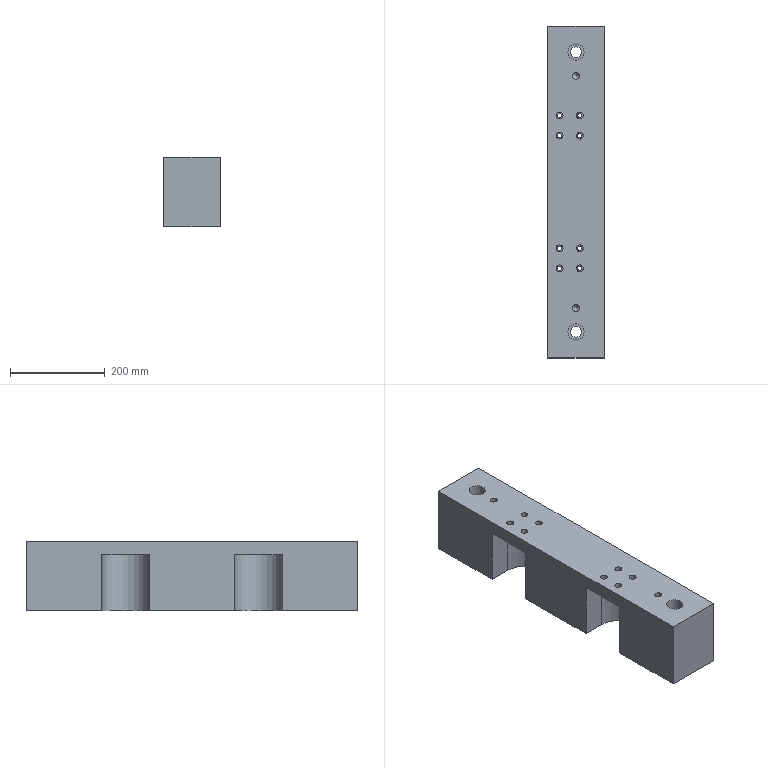Part | STEP file | lll_id2466_x_t | 1 solid | 48 faces | box 120 x 700 x 147.5 mm | volume 10097568 mm3 | cylinder 24 | plane 22 | cone 2 | commonest cylinder face diameters 9.009 x8 14.508 x8 14.506 x2 23.009 x2 34.008 x2 100 x2
STEP:
#1=CARTESIAN_POINT('',(1753.439,295.,370.));
#2=VERTEX_POINT('',#1);
#3=CARTESIAN_POINT('',(1736.435,295.,370.));
#4=DIRECTION('',(0.,0.,-1.));
#5=DIRECTION('',(1.,0.,0.));
#6=AXIS2_PLACEMENT_3D('',#3,#4,#5);
#7=CIRCLE('',#6,17.004);
#8=EDGE_CURVE('',#2,#2,#7,.T.);
#9=ORIENTED_EDGE('',*,*,#8,.T.);
#10=EDGE_LOOP('',(#9));
#11=FACE_BOUND('',#10,.T.);
#12=CARTESIAN_POINT('',(1753.439,-295.,370.));
#13=VERTEX_POINT('',#12);
#14=CARTESIAN_POINT('',(1736.435,-295.,370.));
#15=DIRECTION('',(0.,0.,-1.));
#16=DIRECTION('',(1.,0.,0.));
#17=AXIS2_PLACEMENT_3D('',#14,#15,#16);
#18=CIRCLE('',#17,17.004);
#19=EDGE_CURVE('',#13,#13,#18,.T.);
#20=ORIENTED_EDGE('',*,*,#19,.T.);
#21=EDGE_LOOP('',(#20));
#22=FACE_BOUND('',#21,.T.);
#23=CARTESIAN_POINT('',(1709.041,118.787,370.));
#24=VERTEX_POINT('',#23);
#25=CARTESIAN_POINT('',(1701.787,118.787,370.));
#26=DIRECTION('',(0.,0.,-1.));
#27=DIRECTION('',(1.,0.,0.));
#28=AXIS2_PLACEMENT_3D('',#25,#26,#27);
#29=CIRCLE('',#28,7.254);
#30=EDGE_CURVE('',#24,#24,#29,.T.);
#31=ORIENTED_EDGE('',*,*,#30,.T.);
#32=EDGE_LOOP('',(#31));
#33=FACE_BOUND('',#32,.T.);
#34=CARTESIAN_POINT('',(1751.467,118.787,370.));
#35=VERTEX_POINT('',#34);
#36=CARTESIAN_POINT('',(1744.213,118.787,370.));
#37=DIRECTION('',(0.,0.,-1.));
#38=DIRECTION('',(1.,0.,0.));
#39=AXIS2_PLACEMENT_3D('',#36,#37,#38);
#40=CIRCLE('',#39,7.254);
#41=EDGE_CURVE('',#35,#35,#40,.T.);
#42=ORIENTED_EDGE('',*,*,#41,.T.);
#43=EDGE_LOOP('',(#42));
#44=FACE_BOUND('',#43,.T.);
#45=CARTESIAN_POINT('',(1751.467,-118.787,370.));
#46=VERTEX_POINT('',#45);
#47=CARTESIAN_POINT('',(1744.213,-118.787,370.));
#48=DIRECTION('',(0.,0.,-1.));
#49=DIRECTION('',(1.,0.,0.));
#50=AXIS2_PLACEMENT_3D('',#47,#48,#49);
#51=CIRCLE('',#50,7.254);
#52=EDGE_CURVE('',#46,#46,#51,.T.);
#53=ORIENTED_EDGE('',*,*,#52,.T.);
#54=EDGE_LOOP('',(#53));
#55=FACE_BOUND('',#54,.T.);
#56=CARTESIAN_POINT('',(1709.041,-118.787,370.));
#57=VERTEX_POINT('',#56);
#58=CARTESIAN_POINT('',(1701.787,-118.787,370.));
#59=DIRECTION('',(0.,0.,-1.));
#60=DIRECTION('',(1.,0.,0.));
#61=AXIS2_PLACEMENT_3D('',#58,#59,#60);
#62=CIRCLE('',#61,7.254);
#63=EDGE_CURVE('',#57,#57,#62,.T.);
#64=ORIENTED_EDGE('',*,*,#63,.T.);
#65=EDGE_LOOP('',(#64));
#66=FACE_BOUND('',#65,.T.);
#67=CARTESIAN_POINT('',(1751.467,161.213,370.));
#68=VERTEX_POINT('',#67);
#69=CARTESIAN_POINT('',(1744.213,161.213,370.));
#70=DIRECTION('',(0.,0.,-1.));
#71=DIRECTION('',(1.,0.,0.));
#72=AXIS2_PLACEMENT_3D('',#69,#70,#71);
#73=CIRCLE('',#72,7.254);
#74=EDGE_CURVE('',#68,#68,#73,.T.);
#75=ORIENTED_EDGE('',*,*,#74,.T.);
#76=EDGE_LOOP('',(#75));
#77=FACE_BOUND('',#76,.T.);
#78=CARTESIAN_POINT('',(1709.041,-161.213,370.));
#79=VERTEX_POINT('',#78);
#80=CARTESIAN_POINT('',(1701.787,-161.213,370.));
#81=DIRECTION('',(0.,0.,-1.));
#82=DIRECTION('',(1.,0.,0.));
#83=AXIS2_PLACEMENT_3D('',#80,#81,#82);
#84=CIRCLE('',#83,7.254);
#85=EDGE_CURVE('',#79,#79,#84,.T.);
#86=ORIENTED_EDGE('',*,*,#85,.T.);
#87=EDGE_LOOP('',(#86));
#88=FACE_BOUND('',#87,.T.);
#89=CARTESIAN_POINT('',(1751.467,-161.213,370.));
#90=VERTEX_POINT('',#89);
#91=CARTESIAN_POINT('',(1744.213,-161.213,370.));
#92=DIRECTION('',(0.,0.,-1.));
#93=DIRECTION('',(1.,0.,0.));
#94=AXIS2_PLACEMENT_3D('',#91,#92,#93);
#95=CIRCLE('',#94,7.254);
#96=EDGE_CURVE('',#90,#90,#95,.T.);
#97=ORIENTED_EDGE('',*,*,#96,.T.);
#98=EDGE_LOOP('',(#97));
#99=FACE_BOUND('',#98,.T.);
#100=CARTESIAN_POINT('',(1709.041,161.213,370.));
#101=VERTEX_POINT('',#100);
#102=CARTESIAN_POINT('',(1701.787,161.213,370.));
#103=DIRECTION('',(0.,0.,-1.));
#104=DIRECTION('',(1.,0.,0.));
#105=AXIS2_PLACEMENT_3D('',#102,#103,#104);
#106=CIRCLE('',#105,7.254);
#107=EDGE_CURVE('',#101,#101,#106,.T.);
#108=ORIENTED_EDGE('',*,*,#107,.T.);
#109=EDGE_LOOP('',(#108));
#110=FACE_BOUND('',#109,.T.);
#111=CARTESIAN_POINT('',(1796.435,-350.,370.));
#112=VERTEX_POINT('',#111);
#113=CARTESIAN_POINT('',(1676.435,-350.,370.));
#114=VERTEX_POINT('',#113);
#115=CARTESIAN_POINT('',(3982.751,-350.,370.));
#116=DIRECTION('',(-1.,0.,0.));
#117=VECTOR('',#116,1.);
#118=LINE('',#115,#117);
#119=EDGE_CURVE('',#112,#114,#118,.T.);
#120=ORIENTED_EDGE('',*,*,#119,.F.);
#121=CARTESIAN_POINT('',(1796.435,350.,370.));
#122=VERTEX_POINT('',#121);
#123=CARTESIAN_POINT('',(1796.435,1.,370.));
#124=DIRECTION('',(0.,-1.,0.));
#125=VECTOR('',#124,1.);
#126=LINE('',#123,#125);
#127=EDGE_CURVE('',#122,#112,#126,.T.);
#128=ORIENTED_EDGE('',*,*,#127,.F.);
#129=CARTESIAN_POINT('',(1676.435,350.,370.));
#130=VERTEX_POINT('',#129);
#131=CARTESIAN_POINT('',(3982.751,350.,370.));
#132=DIRECTION('',(1.,0.,0.));
#133=VECTOR('',#132,1.);
#134=LINE('',#131,#133);
#135=EDGE_CURVE('',#130,#122,#134,.T.);
#136=ORIENTED_EDGE('',*,*,#135,.F.);
#137=CARTESIAN_POINT('',(1676.435,0.,370.));
#138=DIRECTION('',(0.,1.,0.));
#139=VECTOR('',#138,1.);
#140=LINE('',#137,#139);
#141=EDGE_CURVE('',#114,#130,#140,.T.);
#142=ORIENTED_EDGE('',*,*,#141,.F.);
#143=EDGE_LOOP('',(#120,#128,#136,#142));
#144=FACE_BOUND('',#143,.T.);
#145=CARTESIAN_POINT('',(1743.688,-245.,370.));
#146=VERTEX_POINT('',#145);
#147=CARTESIAN_POINT('',(1736.435,-245.,370.));
#148=DIRECTION('',(0.,0.,-1.));
#149=DIRECTION('',(1.,0.,0.));
#150=AXIS2_PLACEMENT_3D('',#147,#148,#149);
#151=CIRCLE('',#150,7.253);
#152=EDGE_CURVE('',#146,#146,#151,.T.);
#153=ORIENTED_EDGE('',*,*,#152,.T.);
#154=EDGE_LOOP('',(#153));
#155=FACE_BOUND('',#154,.T.);
#156=CARTESIAN_POINT('',(1743.688,245.,370.));
#157=VERTEX_POINT('',#156);
#158=CARTESIAN_POINT('',(1736.435,245.,370.));
#159=DIRECTION('',(0.,0.,1.));
#160=DIRECTION('',(1.,0.,0.));
#161=AXIS2_PLACEMENT_3D('',#158,#159,#160);
#162=CIRCLE('',#161,7.253);
#163=EDGE_CURVE('',#157,#157,#162,.T.);
#164=ORIENTED_EDGE('',*,*,#163,.F.);
#165=EDGE_LOOP('',(#164));
#166=FACE_BOUND('',#165,.T.);
#167=CARTESIAN_POINT('',(3982.751,1.,370.));
#168=DIRECTION('',(0.,0.,-1.));
#169=DIRECTION('',(-1.,0.,0.));
#170=AXIS2_PLACEMENT_3D('',#167,#168,#169);
#171=PLANE('',#170);
#172=ADVANCED_FACE('',(#11,#22,#33,#44,#55,#66,#77,#88,#99,#110,#144,#155,#166),#171,.F.);
#173=CARTESIAN_POINT('',(1706.291,161.213,341.));
#174=VERTEX_POINT('',#173);
#175=CARTESIAN_POINT('',(1701.787,161.213,341.));
#176=DIRECTION('',(0.,0.,1.));
#177=DIRECTION('',(1.,0.,0.));
#178=AXIS2_PLACEMENT_3D('',#175,#176,#177);
#179=CIRCLE('',#178,4.505);
#180=EDGE_CURVE('',#174,#174,#179,.T.);
#181=ORIENTED_EDGE('',*,*,#180,.T.);
#182=EDGE_LOOP('',(#181));
#183=FACE_BOUND('',#182,.T.);
#184=CARTESIAN_POINT('',(1748.718,161.213,341.));
#185=VERTEX_POINT('',#184);
#186=CARTESIAN_POINT('',(1744.213,161.213,341.));
#187=DIRECTION('',(0.,0.,1.));
#188=DIRECTION('',(1.,0.,0.));
#189=AXIS2_PLACEMENT_3D('',#186,#187,#188);
#190=CIRCLE('',#189,4.505);
#191=EDGE_CURVE('',#185,#185,#190,.T.);
#192=ORIENTED_EDGE('',*,*,#191,.T.);
#193=EDGE_LOOP('',(#192));
#194=FACE_BOUND('',#193,.T.);
#195=CARTESIAN_POINT('',(1748.718,118.787,341.));
#196=VERTEX_POINT('',#195);
#197=CARTESIAN_POINT('',(1744.213,118.787,341.));
#198=DIRECTION('',(0.,0.,1.));
#199=DIRECTION('',(1.,0.,0.));
#200=AXIS2_PLACEMENT_3D('',#197,#198,#199);
#201=CIRCLE('',#200,4.505);
#202=EDGE_CURVE('',#196,#196,#201,.T.);
#203=ORIENTED_EDGE('',*,*,#202,.T.);
#204=EDGE_LOOP('',(#203));
#205=FACE_BOUND('',#204,.T.);
#206=CARTESIAN_POINT('',(1706.291,118.787,341.));
#207=VERTEX_POINT('',#206);
#208=CARTESIAN_POINT('',(1701.787,118.787,341.));
#209=DIRECTION('',(0.,0.,1.));
#210=DIRECTION('',(1.,0.,0.));
#211=AXIS2_PLACEMENT_3D('',#208,#209,#210);
#212=CIRCLE('',#211,4.505);
#213=EDGE_CURVE('',#207,#207,#212,.T.);
#214=ORIENTED_EDGE('',*,*,#213,.T.);
#215=EDGE_LOOP('',(#214));
#216=FACE_BOUND('',#215,.T.);
#217=CARTESIAN_POINT('',(1723.,190.,341.));
#218=VERTEX_POINT('',#217);
#219=CARTESIAN_POINT('',(1676.435,190.,341.));
#220=VERTEX_POINT('',#219);
#221=CARTESIAN_POINT('',(1723.,190.,341.));
#222=DIRECTION('',(-1.,0.,0.));
#223=VECTOR('',#222,1.);
#224=LINE('',#221,#223);
#225=EDGE_CURVE('',#218,#220,#224,.T.);
#226=ORIENTED_EDGE('',*,*,#225,.F.);
#227=CARTESIAN_POINT('',(1723.,90.,341.));
#228=VERTEX_POINT('',#227);
#229=CARTESIAN_POINT('',(1723.,140.,341.));
#230=DIRECTION('',(0.,0.,1.));
#231=DIRECTION('',(1.,0.,0.));
#232=AXIS2_PLACEMENT_3D('',#229,#230,#231);
#233=CIRCLE('',#232,50.);
#234=EDGE_CURVE('',#228,#218,#233,.T.);
#235=ORIENTED_EDGE('',*,*,#234,.F.);
#236=CARTESIAN_POINT('',(1676.435,90.,341.));
#237=VERTEX_POINT('',#236);
#238=CARTESIAN_POINT('',(1723.,90.,341.));
#239=DIRECTION('',(-1.,0.,0.));
#240=VECTOR('',#239,1.);
#241=LINE('',#238,#240);
#242=EDGE_CURVE('',#228,#237,#241,.T.);
#243=ORIENTED_EDGE('',*,*,#242,.T.);
#244=CARTESIAN_POINT('',(1676.435,0.,341.));
#245=DIRECTION('',(0.,-1.,0.));
#246=VECTOR('',#245,1.);
#247=LINE('',#244,#246);
#248=EDGE_CURVE('',#220,#237,#247,.T.);
#249=ORIENTED_EDGE('',*,*,#248,.F.);
#250=EDGE_LOOP('',(#226,#235,#243,#249));
#251=FACE_BOUND('',#250,.T.);
#252=CARTESIAN_POINT('',(1723.,140.,341.));
#253=DIRECTION('',(0.,0.,1.));
#254=DIRECTION('',(1.,0.,0.));
#255=AXIS2_PLACEMENT_3D('',#252,#253,#254);
#256=PLANE('',#255);
#257=ADVANCED_FACE('',(#183,#194,#205,#216,#251),#256,.F.);
#258=CARTESIAN_POINT('',(1748.718,-161.213,341.));
#259=VERTEX_POINT('',#258);
#260=CARTESIAN_POINT('',(1744.213,-161.213,341.));
#261=DIRECTION('',(0.,0.,1.));
#262=DIRECTION('',(1.,0.,0.));
#263=AXIS2_PLACEMENT_3D('',#260,#261,#262);
#264=CIRCLE('',#263,4.505);
#265=EDGE_CURVE('',#259,#259,#264,.T.);
#266=ORIENTED_EDGE('',*,*,#265,.T.);
#267=EDGE_LOOP('',(#266));
#268=FACE_BOUND('',#267,.T.);
#269=CARTESIAN_POINT('',(1706.291,-161.213,341.));
#270=VERTEX_POINT('',#269);
#271=CARTESIAN_POINT('',(1701.787,-161.213,341.));
#272=DIRECTION('',(0.,0.,1.));
#273=DIRECTION('',(1.,0.,0.));
#274=AXIS2_PLACEMENT_3D('',#271,#272,#273);
#275=CIRCLE('',#274,4.505);
#276=EDGE_CURVE('',#270,#270,#275,.T.);
#277=ORIENTED_EDGE('',*,*,#276,.T.);
#278=EDGE_LOOP('',(#277));
#279=FACE_BOUND('',#278,.T.);
#280=CARTESIAN_POINT('',(1706.291,-118.787,341.));
#281=VERTEX_POINT('',#280);
#282=CARTESIAN_POINT('',(1701.787,-118.787,341.));
#283=DIRECTION('',(0.,0.,1.));
#284=DIRECTION('',(1.,0.,0.));
#285=AXIS2_PLACEMENT_3D('',#282,#283,#284);
#286=CIRCLE('',#285,4.505);
#287=EDGE_CURVE('',#281,#281,#286,.T.);
#288=ORIENTED_EDGE('',*,*,#287,.T.);
#289=EDGE_LOOP('',(#288));
#290=FACE_BOUND('',#289,.T.);
#291=CARTESIAN_POINT('',(1748.718,-118.787,341.));
#292=VERTEX_POINT('',#291);
#293=CARTESIAN_POINT('',(1744.213,-118.787,341.));
#294=DIRECTION('',(0.,0.,1.));
#295=DIRECTION('',(1.,0.,0.));
#296=AXIS2_PLACEMENT_3D('',#293,#294,#295);
#297=CIRCLE('',#296,4.505);
#298=EDGE_CURVE('',#292,#292,#297,.T.);
#299=ORIENTED_EDGE('',*,*,#298,.T.);
#300=EDGE_LOOP('',(#299));
#301=FACE_BOUND('',#300,.T.);
#302=CARTESIAN_POINT('',(1723.,-90.,341.));
#303=VERTEX_POINT('',#302);
#304=CARTESIAN_POINT('',(1676.435,-90.,341.));
#305=VERTEX_POINT('',#304);
#306=CARTESIAN_POINT('',(1723.,-90.,341.));
#307=DIRECTION('',(-1.,0.,0.));
#308=VECTOR('',#307,1.);
#309=LINE('',#306,#308);
#310=EDGE_CURVE('',#303,#305,#309,.T.);
#311=ORIENTED_EDGE('',*,*,#310,.F.);
#312=CARTESIAN_POINT('',(1723.,-190.,341.));
#313=VERTEX_POINT('',#312);
#314=CARTESIAN_POINT('',(1723.,-140.,341.));
#315=DIRECTION('',(0.,0.,1.));
#316=DIRECTION('',(1.,0.,0.));
#317=AXIS2_PLACEMENT_3D('',#314,#315,#316);
#318=CIRCLE('',#317,50.);
#319=EDGE_CURVE('',#313,#303,#318,.T.);
#320=ORIENTED_EDGE('',*,*,#319,.F.);
#321=CARTESIAN_POINT('',(1676.435,-190.,341.));
#322=VERTEX_POINT('',#321);
#323=CARTESIAN_POINT('',(1723.,-190.,341.));
#324=DIRECTION('',(-1.,0.,0.));
#325=VECTOR('',#324,1.);
#326=LINE('',#323,#325);
#327=EDGE_CURVE('',#313,#322,#326,.T.);
#328=ORIENTED_EDGE('',*,*,#327,.T.);
#329=CARTESIAN_POINT('',(1676.435,0.,341.));
#330=DIRECTION('',(0.,-1.,0.));
#331=VECTOR('',#330,1.);
#332=LINE('',#329,#331);
#333=EDGE_CURVE('',#305,#322,#332,.T.);
#334=ORIENTED_EDGE('',*,*,#333,.F.);
#335=EDGE_LOOP('',(#311,#320,#328,#334));
#336=FACE_BOUND('',#335,.T.);
#337=CARTESIAN_POINT('',(1723.,140.,341.));
#338=DIRECTION('',(0.,0.,1.));
#339=DIRECTION('',(1.,0.,0.));
#340=AXIS2_PLACEMENT_3D('',#337,#338,#339);
#341=PLANE('',#340);
#342=ADVANCED_FACE('',(#268,#279,#290,#301,#336),#341,.F.);
#343=CARTESIAN_POINT('',(1796.435,-350.,222.5));
#344=VERTEX_POINT('',#343);
#345=CARTESIAN_POINT('',(1796.435,-350.,310.));
#346=DIRECTION('',(0.,0.,-1.));
#347=VECTOR('',#346,1.);
#348=LINE('',#345,#347);
#349=EDGE_CURVE('',#112,#344,#348,.T.);
#350=ORIENTED_EDGE('',*,*,#349,.T.);
#351=CARTESIAN_POINT('',(1796.435,350.,222.5));
#352=VERTEX_POINT('',#351);
#353=CARTESIAN_POINT('',(1796.435,600.,222.5));
#354=DIRECTION('',(0.,-1.,0.));
#355=VECTOR('',#354,1.);
#356=LINE('',#353,#355);
#357=EDGE_CURVE('',#352,#344,#356,.T.);
#358=ORIENTED_EDGE('',*,*,#357,.F.);
#359=CARTESIAN_POINT('',(1796.435,350.,310.));
#360=DIRECTION('',(0.,0.,-1.));
#361=VECTOR('',#360,1.);
#362=LINE('',#359,#361);
#363=EDGE_CURVE('',#122,#352,#362,.T.);
#364=ORIENTED_EDGE('',*,*,#363,.F.);
#365=ORIENTED_EDGE('',*,*,#127,.T.);
#366=EDGE_LOOP('',(#350,#358,#364,#365));
#367=FACE_OUTER_BOUND('',#366,.T.);
#368=CARTESIAN_POINT('',(1796.435,600.,310.));
#369=DIRECTION('',(1.,0.,0.));
#370=DIRECTION('',(0.,0.,-1.));
#371=AXIS2_PLACEMENT_3D('',#368,#369,#370);
#372=PLANE('',#371);
#373=ADVANCED_FACE('',(#367),#372,.T.);
#374=CARTESIAN_POINT('',(1676.435,-350.,222.5));
#375=VERTEX_POINT('',#374);
#376=CARTESIAN_POINT('',(1676.435,-350.,241.25));
#377=DIRECTION('',(0.,0.,-1.));
#378=VECTOR('',#377,1.);
#379=LINE('',#376,#378);
#380=EDGE_CURVE('',#114,#375,#379,.T.);
#381=ORIENTED_EDGE('',*,*,#380,.T.);
#382=CARTESIAN_POINT('',(3982.751,-350.,222.5));
#383=DIRECTION('',(-1.,0.,0.));
#384=VECTOR('',#383,1.);
#385=LINE('',#382,#384);
#386=EDGE_CURVE('',#344,#375,#385,.T.);
#387=ORIENTED_EDGE('',*,*,#386,.F.);
#388=ORIENTED_EDGE('',*,*,#349,.F.);
#389=ORIENTED_EDGE('',*,*,#119,.T.);
#390=EDGE_LOOP('',(#381,#387,#388,#389));
#391=FACE_OUTER_BOUND('',#390,.T.);
#392=CARTESIAN_POINT('',(1796.435,-350.,310.));
#393=DIRECTION('',(0.,-1.,0.));
#394=DIRECTION('',(0.,0.,-1.));
#395=AXIS2_PLACEMENT_3D('',#392,#393,#394);
#396=PLANE('',#395);
#397=ADVANCED_FACE('',(#391),#396,.T.);
#398=ORIENTED_EDGE('',*,*,#363,.T.);
#399=CARTESIAN_POINT('',(1676.435,350.,222.5));
#400=VERTEX_POINT('',#399);
#401=CARTESIAN_POINT('',(3982.751,350.,222.5));
#402=DIRECTION('',(1.,0.,0.));
#403=VECTOR('',#402,1.);
#404=LINE('',#401,#403);
#405=EDGE_CURVE('',#400,#352,#404,.T.);
#406=ORIENTED_EDGE('',*,*,#405,.F.);
#407=CARTESIAN_POINT('',(1676.435,350.,241.25));
#408=DIRECTION('',(0.,0.,1.));
#409=VECTOR('',#408,1.);
#410=LINE('',#407,#409);
#411=EDGE_CURVE('',#400,#130,#410,.T.);
#412=ORIENTED_EDGE('',*,*,#411,.T.);
#413=ORIENTED_EDGE('',*,*,#135,.T.);
#414=EDGE_LOOP('',(#398,#406,#412,#413));
#415=FACE_OUTER_BOUND('',#414,.T.);
#416=CARTESIAN_POINT('',(-2173.565,350.,310.));
#417=DIRECTION('',(0.,1.,0.));
#418=DIRECTION('',(0.,0.,1.));
#419=AXIS2_PLACEMENT_3D('',#416,#417,#418);
#420=PLANE('',#419);
#421=ADVANCED_FACE('',(#415),#420,.T.);
#422=ORIENTED_EDGE('',*,*,#411,.F.);
#423=CARTESIAN_POINT('',(1676.435,190.,222.5));
#424=VERTEX_POINT('',#423);
#425=CARTESIAN_POINT('',(1676.435,1.,222.5));
#426=DIRECTION('',(0.,-1.,0.));
#427=VECTOR('',#426,1.);
#428=LINE('',#425,#427);
#429=EDGE_CURVE('',#400,#424,#428,.T.);
#430=ORIENTED_EDGE('',*,*,#429,.T.);
#431=CARTESIAN_POINT('',(1676.435,190.,241.25));
#432=DIRECTION('',(0.,0.,-1.));
#433=VECTOR('',#432,1.);
#434=LINE('',#431,#433);
#435=EDGE_CURVE('',#220,#424,#434,.T.);
#436=ORIENTED_EDGE('',*,*,#435,.F.);
#437=ORIENTED_EDGE('',*,*,#248,.T.);
#438=CARTESIAN_POINT('',(1676.435,90.,222.5));
#439=VERTEX_POINT('',#438);
#440=CARTESIAN_POINT('',(1676.435,90.,241.25));
#441=DIRECTION('',(0.,0.,-1.));
#442=VECTOR('',#441,1.);
#443=LINE('',#440,#442);
#444=EDGE_CURVE('',#237,#439,#443,.T.);
#445=ORIENTED_EDGE('',*,*,#444,.T.);
#446=CARTESIAN_POINT('',(1676.435,-90.,222.5));
#447=VERTEX_POINT('',#446);
#448=CARTESIAN_POINT('',(1676.435,1.,222.5));
#449=DIRECTION('',(0.,-1.,0.));
#450=VECTOR('',#449,1.);
#451=LINE('',#448,#450);
#452=EDGE_CURVE('',#439,#447,#451,.T.);
#453=ORIENTED_EDGE('',*,*,#452,.T.);
#454=CARTESIAN_POINT('',(1676.435,-90.,241.25));
#455=DIRECTION('',(0.,0.,-1.));
#456=VECTOR('',#455,1.);
#457=LINE('',#454,#456);
#458=EDGE_CURVE('',#305,#447,#457,.T.);
#459=ORIENTED_EDGE('',*,*,#458,.F.);
#460=ORIENTED_EDGE('',*,*,#333,.T.);
#461=CARTESIAN_POINT('',(1676.435,-190.,222.5));
#462=VERTEX_POINT('',#461);
#463=CARTESIAN_POINT('',(1676.435,-190.,241.25));
#464=DIRECTION('',(0.,0.,1.));
#465=VECTOR('',#464,1.);
#466=LINE('',#463,#465);
#467=EDGE_CURVE('',#462,#322,#466,.T.);
#468=ORIENTED_EDGE('',*,*,#467,.F.);
#469=CARTESIAN_POINT('',(1676.435,1.,222.5));
#470=DIRECTION('',(0.,-1.,0.));
#471=VECTOR('',#470,1.);
#472=LINE('',#469,#471);
#473=EDGE_CURVE('',#462,#375,#472,.T.);
#474=ORIENTED_EDGE('',*,*,#473,.T.);
#475=ORIENTED_EDGE('',*,*,#380,.F.);
#476=ORIENTED_EDGE('',*,*,#141,.T.);
#477=EDGE_LOOP('',(#422,#430,#436,#437,#445,#453,#459,#460,#468,#474,#475,#476));
#478=FACE_OUTER_BOUND('',#477,.T.);
#479=CARTESIAN_POINT('',(1676.435,0.,241.25));
#480=DIRECTION('',(1.,0.,0.));
#481=DIRECTION('',(0.,0.,-1.));
#482=AXIS2_PLACEMENT_3D('',#479,#480,#481);
#483=PLANE('',#482);
#484=ADVANCED_FACE('',(#478),#483,.F.);
#485=CARTESIAN_POINT('',(1697.282,161.213,356.));
#486=VERTEX_POINT('',#485);
#487=CARTESIAN_POINT('',(1701.787,161.213,356.));
#488=DIRECTION('',(0.,0.,-1.));
#489=DIRECTION('',(-1.,0.,0.));
#490=AXIS2_PLACEMENT_3D('',#487,#488,#489);
#491=CIRCLE('',#490,4.505);
#492=EDGE_CURVE('',#486,#486,#491,.T.);
#493=ORIENTED_EDGE('',*,*,#492,.F.);
#494=EDGE_LOOP('',(#493));
#495=FACE_BOUND('',#494,.T.);
#496=ORIENTED_EDGE('',*,*,#180,.F.);
#497=EDGE_LOOP('',(#496));
#498=FACE_BOUND('',#497,.T.);
#499=CARTESIAN_POINT('',(1701.787,161.213,370.));
#500=DIRECTION('',(0.,0.,-1.));
#501=DIRECTION('',(1.,0.,0.));
#502=AXIS2_PLACEMENT_3D('',#499,#500,#501);
#503=CYLINDRICAL_SURFACE('',#502,4.505);
#504=ADVANCED_FACE('',(#495,#498),#503,.F.);
#505=ORIENTED_EDGE('',*,*,#492,.T.);
#506=EDGE_LOOP('',(#505));
#507=FACE_BOUND('',#506,.T.);
#508=CARTESIAN_POINT('',(1709.041,161.213,356.));
#509=VERTEX_POINT('',#508);
#510=CARTESIAN_POINT('',(1701.787,161.213,356.));
#511=DIRECTION('',(0.,0.,-1.));
#512=DIRECTION('',(1.,0.,0.));
#513=AXIS2_PLACEMENT_3D('',#510,#511,#512);
#514=CIRCLE('',#513,7.254);
#515=EDGE_CURVE('',#509,#509,#514,.T.);
#516=ORIENTED_EDGE('',*,*,#515,.F.);
#517=EDGE_LOOP('',(#516));
#518=FACE_BOUND('',#517,.T.);
#519=CARTESIAN_POINT('',(1701.787,161.213,356.));
#520=DIRECTION('',(0.,0.,-1.));
#521=DIRECTION('',(-1.,0.,0.));
#522=AXIS2_PLACEMENT_3D('',#519,#520,#521);
#523=PLANE('',#522);
#524=ADVANCED_FACE('',(#507,#518),#523,.F.);
#525=ORIENTED_EDGE('',*,*,#515,.T.);
#526=EDGE_LOOP('',(#525));
#527=FACE_BOUND('',#526,.T.);
#528=ORIENTED_EDGE('',*,*,#107,.F.);
#529=EDGE_LOOP('',(#528));
#530=FACE_BOUND('',#529,.T.);
#531=CARTESIAN_POINT('',(1701.787,161.213,370.));
#532=DIRECTION('',(0.,0.,-1.));
#533=DIRECTION('',(1.,0.,0.));
#534=AXIS2_PLACEMENT_3D('',#531,#532,#533);
#535=CYLINDRICAL_SURFACE('',#534,7.254);
#536=ADVANCED_FACE('',(#527,#530),#535,.F.);
#537=CARTESIAN_POINT('',(1739.709,-161.213,356.));
#538=VERTEX_POINT('',#537);
#539=CARTESIAN_POINT('',(1744.213,-161.213,356.));
#540=DIRECTION('',(0.,0.,-1.));
#541=DIRECTION('',(-1.,0.,0.));
#542=AXIS2_PLACEMENT_3D('',#539,#540,#541);
#543=CIRCLE('',#542,4.505);
#544=EDGE_CURVE('',#538,#538,#543,.T.);
#545=ORIENTED_EDGE('',*,*,#544,.F.);
#546=EDGE_LOOP('',(#545));
#547=FACE_BOUND('',#546,.T.);
#548=ORIENTED_EDGE('',*,*,#265,.F.);
#549=EDGE_LOOP('',(#548));
#550=FACE_BOUND('',#549,.T.);
#551=CARTESIAN_POINT('',(1744.213,-161.213,370.));
#552=DIRECTION('',(0.,0.,-1.));
#553=DIRECTION('',(1.,0.,0.));
#554=AXIS2_PLACEMENT_3D('',#551,#552,#553);
#555=CYLINDRICAL_SURFACE('',#554,4.505);
#556=ADVANCED_FACE('',(#547,#550),#555,.F.);
#557=ORIENTED_EDGE('',*,*,#544,.T.);
#558=EDGE_LOOP('',(#557));
#559=FACE_BOUND('',#558,.T.);
#560=CARTESIAN_POINT('',(1751.467,-161.213,356.));
#561=VERTEX_POINT('',#560);
#562=CARTESIAN_POINT('',(1744.213,-161.213,356.));
#563=DIRECTION('',(0.,0.,-1.));
#564=DIRECTION('',(1.,0.,0.));
#565=AXIS2_PLACEMENT_3D('',#562,#563,#564);
#566=CIRCLE('',#565,7.254);
#567=EDGE_CURVE('',#561,#561,#566,.T.);
#568=ORIENTED_EDGE('',*,*,#567,.F.);
#569=EDGE_LOOP('',(#568));
#570=FACE_BOUND('',#569,.T.);
#571=CARTESIAN_POINT('',(1744.213,-161.213,356.));
#572=DIRECTION('',(0.,0.,-1.));
#573=DIRECTION('',(-1.,0.,0.));
#574=AXIS2_PLACEMENT_3D('',#571,#572,#573);
#575=PLANE('',#574);
#576=ADVANCED_FACE('',(#559,#570),#575,.F.);
#577=ORIENTED_EDGE('',*,*,#567,.T.);
#578=EDGE_LOOP('',(#577));
#579=FACE_BOUND('',#578,.T.);
#580=ORIENTED_EDGE('',*,*,#96,.F.);
#581=EDGE_LOOP('',(#580));
#582=FACE_BOUND('',#581,.T.);
#583=CARTESIAN_POINT('',(1744.213,-161.213,370.));
#584=DIRECTION('',(0.,0.,-1.));
#585=DIRECTION('',(1.,0.,0.));
#586=AXIS2_PLACEMENT_3D('',#583,#584,#585);
#587=CYLINDRICAL_SURFACE('',#586,7.254);
#588=ADVANCED_FACE('',(#579,#582),#587,.F.);
#589=CARTESIAN_POINT('',(1697.282,-161.213,356.));
#590=VERTEX_POINT('',#589);
#591=CARTESIAN_POINT('',(1701.787,-161.213,356.));
#592=DIRECTION('',(0.,0.,-1.));
#593=DIRECTION('',(-1.,0.,0.));
#594=AXIS2_PLACEMENT_3D('',#591,#592,#593);
#595=CIRCLE('',#594,4.505);
#596=EDGE_CURVE('',#590,#590,#595,.T.);
#597=ORIENTED_EDGE('',*,*,#596,.F.);
#598=EDGE_LOOP('',(#597));
#599=FACE_BOUND('',#598,.T.);
#600=ORIENTED_EDGE('',*,*,#276,.F.);
#601=EDGE_LOOP('',(#600));
#602=FACE_BOUND('',#601,.T.);
#603=CARTESIAN_POINT('',(1701.787,-161.213,370.));
#604=DIRECTION('',(0.,0.,-1.));
#605=DIRECTION('',(1.,0.,0.));
#606=AXIS2_PLACEMENT_3D('',#603,#604,#605);
#607=CYLINDRICAL_SURFACE('',#606,4.505);
#608=ADVANCED_FACE('',(#599,#602),#607,.F.);
#609=ORIENTED_EDGE('',*,*,#596,.T.);
#610=EDGE_LOOP('',(#609));
#611=FACE_BOUND('',#610,.T.);
#612=CARTESIAN_POINT('',(1709.041,-161.213,356.));
#613=VERTEX_POINT('',#612);
#614=CARTESIAN_POINT('',(1701.787,-161.213,356.));
#615=DIRECTION('',(0.,0.,-1.));
#616=DIRECTION('',(1.,0.,0.));
#617=AXIS2_PLACEMENT_3D('',#614,#615,#616);
#618=CIRCLE('',#617,7.254);
#619=EDGE_CURVE('',#613,#613,#618,.T.);
#620=ORIENTED_EDGE('',*,*,#619,.F.);
#621=EDGE_LOOP('',(#620));
#622=FACE_BOUND('',#621,.T.);
#623=CARTESIAN_POINT('',(1701.787,-161.213,356.));
#624=DIRECTION('',(0.,0.,-1.));
#625=DIRECTION('',(-1.,0.,0.));
#626=AXIS2_PLACEMENT_3D('',#623,#624,#625);
#627=PLANE('',#626);
#628=ADVANCED_FACE('',(#611,#622),#627,.F.);
#629=ORIENTED_EDGE('',*,*,#619,.T.);
#630=EDGE_LOOP('',(#629));
#631=FACE_BOUND('',#630,.T.);
#632=ORIENTED_EDGE('',*,*,#85,.F.);
#633=EDGE_LOOP('',(#632));
#634=FACE_BOUND('',#633,.T.);
#635=CARTESIAN_POINT('',(1701.787,-161.213,370.));
#636=DIRECTION('',(0.,0.,-1.));
#637=DIRECTION('',(1.,0.,0.));
#638=AXIS2_PLACEMENT_3D('',#635,#636,#637);
#639=CYLINDRICAL_SURFACE('',#638,7.254);
#640=ADVANCED_FACE('',(#631,#634),#639,.F.);
#641=CARTESIAN_POINT('',(1739.709,161.213,356.));
#642=VERTEX_POINT('',#641);
#643=CARTESIAN_POINT('',(1744.213,161.213,356.));
#644=DIRECTION('',(0.,0.,-1.));
#645=DIRECTION('',(-1.,0.,0.));
#646=AXIS2_PLACEMENT_3D('',#643,#644,#645);
#647=CIRCLE('',#646,4.505);
#648=EDGE_CURVE('',#642,#642,#647,.T.);
#649=ORIENTED_EDGE('',*,*,#648,.F.);
#650=EDGE_LOOP('',(#649));
#651=FACE_BOUND('',#650,.T.);
#652=ORIENTED_EDGE('',*,*,#191,.F.);
#653=EDGE_LOOP('',(#652));
#654=FACE_BOUND('',#653,.T.);
#655=CARTESIAN_POINT('',(1744.213,161.213,370.));
#656=DIRECTION('',(0.,0.,-1.));
#657=DIRECTION('',(1.,0.,0.));
#658=AXIS2_PLACEMENT_3D('',#655,#656,#657);
#659=CYLINDRICAL_SURFACE('',#658,4.505);
#660=ADVANCED_FACE('',(#651,#654),#659,.F.);
#661=ORIENTED_EDGE('',*,*,#648,.T.);
#662=EDGE_LOOP('',(#661));
#663=FACE_BOUND('',#662,.T.);
#664=CARTESIAN_POINT('',(1751.467,161.213,356.));
#665=VERTEX_POINT('',#664);
#666=CARTESIAN_POINT('',(1744.213,161.213,356.));
#667=DIRECTION('',(0.,0.,-1.));
#668=DIRECTION('',(1.,0.,0.));
#669=AXIS2_PLACEMENT_3D('',#666,#667,#668);
#670=CIRCLE('',#669,7.254);
#671=EDGE_CURVE('',#665,#665,#670,.T.);
#672=ORIENTED_EDGE('',*,*,#671,.F.);
#673=EDGE_LOOP('',(#672));
#674=FACE_BOUND('',#673,.T.);
#675=CARTESIAN_POINT('',(1744.213,161.213,356.));
#676=DIRECTION('',(0.,0.,-1.));
#677=DIRECTION('',(-1.,0.,0.));
#678=AXIS2_PLACEMENT_3D('',#675,#676,#677);
#679=PLANE('',#678);
#680=ADVANCED_FACE('',(#663,#674),#679,.F.);
#681=ORIENTED_EDGE('',*,*,#671,.T.);
#682=EDGE_LOOP('',(#681));
#683=FACE_BOUND('',#682,.T.);
#684=ORIENTED_EDGE('',*,*,#74,.F.);
#685=EDGE_LOOP('',(#684));
#686=FACE_BOUND('',#685,.T.);
#687=CARTESIAN_POINT('',(1744.213,161.213,370.));
#688=DIRECTION('',(0.,0.,-1.));
#689=DIRECTION('',(1.,0.,0.));
#690=AXIS2_PLACEMENT_3D('',#687,#688,#689);
#691=CYLINDRICAL_SURFACE('',#690,7.254);
#692=ADVANCED_FACE('',(#683,#686),#691,.F.);
#693=CARTESIAN_POINT('',(1697.282,-118.787,356.));
#694=VERTEX_POINT('',#693);
#695=CARTESIAN_POINT('',(1701.787,-118.787,356.));
#696=DIRECTION('',(0.,0.,-1.));
#697=DIRECTION('',(-1.,0.,0.));
#698=AXIS2_PLACEMENT_3D('',#695,#696,#697);
#699=CIRCLE('',#698,4.505);
#700=EDGE_CURVE('',#694,#694,#699,.T.);
#701=ORIENTED_EDGE('',*,*,#700,.F.);
#702=EDGE_LOOP('',(#701));
#703=FACE_BOUND('',#702,.T.);
#704=ORIENTED_EDGE('',*,*,#287,.F.);
#705=EDGE_LOOP('',(#704));
#706=FACE_BOUND('',#705,.T.);
#707=CARTESIAN_POINT('',(1701.787,-118.787,370.));
#708=DIRECTION('',(0.,0.,-1.));
#709=DIRECTION('',(1.,0.,0.));
#710=AXIS2_PLACEMENT_3D('',#707,#708,#709);
#711=CYLINDRICAL_SURFACE('',#710,4.505);
#712=ADVANCED_FACE('',(#703,#706),#711,.F.);
#713=ORIENTED_EDGE('',*,*,#700,.T.);
#714=EDGE_LOOP('',(#713));
#715=FACE_BOUND('',#714,.T.);
#716=CARTESIAN_POINT('',(1709.041,-118.787,356.));
#717=VERTEX_POINT('',#716);
#718=CARTESIAN_POINT('',(1701.787,-118.787,356.));
#719=DIRECTION('',(0.,0.,-1.));
#720=DIRECTION('',(1.,0.,0.));
#721=AXIS2_PLACEMENT_3D('',#718,#719,#720);
#722=CIRCLE('',#721,7.254);
#723=EDGE_CURVE('',#717,#717,#722,.T.);
#724=ORIENTED_EDGE('',*,*,#723,.F.);
#725=EDGE_LOOP('',(#724));
#726=FACE_BOUND('',#725,.T.);
#727=CARTESIAN_POINT('',(1701.787,-118.787,356.));
#728=DIRECTION('',(0.,0.,-1.));
#729=DIRECTION('',(-1.,0.,0.));
#730=AXIS2_PLACEMENT_3D('',#727,#728,#729);
#731=PLANE('',#730);
#732=ADVANCED_FACE('',(#715,#726),#731,.F.);
#733=ORIENTED_EDGE('',*,*,#723,.T.);
#734=EDGE_LOOP('',(#733));
#735=FACE_BOUND('',#734,.T.);
#736=ORIENTED_EDGE('',*,*,#63,.F.);
#737=EDGE_LOOP('',(#736));
#738=FACE_BOUND('',#737,.T.);
#739=CARTESIAN_POINT('',(1701.787,-118.787,370.));
#740=DIRECTION('',(0.,0.,-1.));
#741=DIRECTION('',(1.,0.,0.));
#742=AXIS2_PLACEMENT_3D('',#739,#740,#741);
#743=CYLINDRICAL_SURFACE('',#742,7.254);
#744=ADVANCED_FACE('',(#735,#738),#743,.F.);
#745=CARTESIAN_POINT('',(1739.709,-118.787,356.));
#746=VERTEX_POINT('',#745);
#747=CARTESIAN_POINT('',(1744.213,-118.787,356.));
#748=DIRECTION('',(0.,0.,-1.));
#749=DIRECTION('',(-1.,0.,0.));
#750=AXIS2_PLACEMENT_3D('',#747,#748,#749);
#751=CIRCLE('',#750,4.505);
#752=EDGE_CURVE('',#746,#746,#751,.T.);
#753=ORIENTED_EDGE('',*,*,#752,.F.);
#754=EDGE_LOOP('',(#753));
#755=FACE_BOUND('',#754,.T.);
#756=ORIENTED_EDGE('',*,*,#298,.F.);
#757=EDGE_LOOP('',(#756));
#758=FACE_BOUND('',#757,.T.);
#759=CARTESIAN_POINT('',(1744.213,-118.787,370.));
#760=DIRECTION('',(0.,0.,-1.));
#761=DIRECTION('',(1.,0.,0.));
#762=AXIS2_PLACEMENT_3D('',#759,#760,#761);
#763=CYLINDRICAL_SURFACE('',#762,4.505);
#764=ADVANCED_FACE('',(#755,#758),#763,.F.);
#765=ORIENTED_EDGE('',*,*,#752,.T.);
#766=EDGE_LOOP('',(#765));
#767=FACE_BOUND('',#766,.T.);
#768=CARTESIAN_POINT('',(1751.467,-118.787,356.));
#769=VERTEX_POINT('',#768);
#770=CARTESIAN_POINT('',(1744.213,-118.787,356.));
#771=DIRECTION('',(0.,0.,-1.));
#772=DIRECTION('',(1.,0.,0.));
#773=AXIS2_PLACEMENT_3D('',#770,#771,#772);
#774=CIRCLE('',#773,7.254);
#775=EDGE_CURVE('',#769,#769,#774,.T.);
#776=ORIENTED_EDGE('',*,*,#775,.F.);
#777=EDGE_LOOP('',(#776));
#778=FACE_BOUND('',#777,.T.);
#779=CARTESIAN_POINT('',(1744.213,-118.787,356.));
#780=DIRECTION('',(0.,0.,-1.));
#781=DIRECTION('',(-1.,0.,0.));
#782=AXIS2_PLACEMENT_3D('',#779,#780,#781);
#783=PLANE('',#782);
#784=ADVANCED_FACE('',(#767,#778),#783,.F.);
#785=ORIENTED_EDGE('',*,*,#775,.T.);
#786=EDGE_LOOP('',(#785));
#787=FACE_BOUND('',#786,.T.);
#788=ORIENTED_EDGE('',*,*,#52,.F.);
#789=EDGE_LOOP('',(#788));
#790=FACE_BOUND('',#789,.T.);
#791=CARTESIAN_POINT('',(1744.213,-118.787,370.));
#792=DIRECTION('',(0.,0.,-1.));
#793=DIRECTION('',(1.,0.,0.));
#794=AXIS2_PLACEMENT_3D('',#791,#792,#793);
#795=CYLINDRICAL_SURFACE('',#794,7.254);
#796=ADVANCED_FACE('',(#787,#790),#795,.F.);
#797=CARTESIAN_POINT('',(1739.709,118.787,356.));
#798=VERTEX_POINT('',#797);
#799=CARTESIAN_POINT('',(1744.213,118.787,356.));
#800=DIRECTION('',(0.,0.,-1.));
#801=DIRECTION('',(-1.,0.,0.));
#802=AXIS2_PLACEMENT_3D('',#799,#800,#801);
#803=CIRCLE('',#802,4.505);
#804=EDGE_CURVE('',#798,#798,#803,.T.);
#805=ORIENTED_EDGE('',*,*,#804,.F.);
#806=EDGE_LOOP('',(#805));
#807=FACE_BOUND('',#806,.T.);
#808=ORIENTED_EDGE('',*,*,#202,.F.);
#809=EDGE_LOOP('',(#808));
#810=FACE_BOUND('',#809,.T.);
#811=CARTESIAN_POINT('',(1744.213,118.787,370.));
#812=DIRECTION('',(0.,0.,-1.));
#813=DIRECTION('',(1.,0.,0.));
#814=AXIS2_PLACEMENT_3D('',#811,#812,#813);
#815=CYLINDRICAL_SURFACE('',#814,4.505);
#816=ADVANCED_FACE('',(#807,#810),#815,.F.);
#817=ORIENTED_EDGE('',*,*,#804,.T.);
#818=EDGE_LOOP('',(#817));
#819=FACE_BOUND('',#818,.T.);
#820=CARTESIAN_POINT('',(1751.467,118.787,356.));
#821=VERTEX_POINT('',#820);
#822=CARTESIAN_POINT('',(1744.213,118.787,356.));
#823=DIRECTION('',(0.,0.,-1.));
#824=DIRECTION('',(1.,0.,0.));
#825=AXIS2_PLACEMENT_3D('',#822,#823,#824);
#826=CIRCLE('',#825,7.254);
#827=EDGE_CURVE('',#821,#821,#826,.T.);
#828=ORIENTED_EDGE('',*,*,#827,.F.);
#829=EDGE_LOOP('',(#828));
#830=FACE_BOUND('',#829,.T.);
#831=CARTESIAN_POINT('',(1744.213,118.787,356.));
#832=DIRECTION('',(0.,0.,-1.));
#833=DIRECTION('',(-1.,0.,0.));
#834=AXIS2_PLACEMENT_3D('',#831,#832,#833);
#835=PLANE('',#834);
#836=ADVANCED_FACE('',(#819,#830),#835,.F.);
#837=ORIENTED_EDGE('',*,*,#827,.T.);
#838=EDGE_LOOP('',(#837));
#839=FACE_BOUND('',#838,.T.);
#840=ORIENTED_EDGE('',*,*,#41,.F.);
#841=EDGE_LOOP('',(#840));
#842=FACE_BOUND('',#841,.T.);
#843=CARTESIAN_POINT('',(1744.213,118.787,370.));
#844=DIRECTION('',(0.,0.,-1.));
#845=DIRECTION('',(1.,0.,0.));
#846=AXIS2_PLACEMENT_3D('',#843,#844,#845);
#847=CYLINDRICAL_SURFACE('',#846,7.254);
#848=ADVANCED_FACE('',(#839,#842),#847,.F.);
#849=CARTESIAN_POINT('',(1697.282,118.787,356.));
#850=VERTEX_POINT('',#849);
#851=CARTESIAN_POINT('',(1701.787,118.787,356.));
#852=DIRECTION('',(0.,0.,-1.));
#853=DIRECTION('',(-1.,0.,0.));
#854=AXIS2_PLACEMENT_3D('',#851,#852,#853);
#855=CIRCLE('',#854,4.505);
#856=EDGE_CURVE('',#850,#850,#855,.T.);
#857=ORIENTED_EDGE('',*,*,#856,.F.);
#858=EDGE_LOOP('',(#857));
#859=FACE_BOUND('',#858,.T.);
#860=ORIENTED_EDGE('',*,*,#213,.F.);
#861=EDGE_LOOP('',(#860));
#862=FACE_BOUND('',#861,.T.);
#863=CARTESIAN_POINT('',(1701.787,118.787,370.));
#864=DIRECTION('',(0.,0.,-1.));
#865=DIRECTION('',(1.,0.,0.));
#866=AXIS2_PLACEMENT_3D('',#863,#864,#865);
#867=CYLINDRICAL_SURFACE('',#866,4.505);
#868=ADVANCED_FACE('',(#859,#862),#867,.F.);
#869=ORIENTED_EDGE('',*,*,#856,.T.);
#870=EDGE_LOOP('',(#869));
#871=FACE_BOUND('',#870,.T.);
#872=CARTESIAN_POINT('',(1709.041,118.787,356.));
#873=VERTEX_POINT('',#872);
#874=CARTESIAN_POINT('',(1701.787,118.787,356.));
#875=DIRECTION('',(0.,0.,-1.));
#876=DIRECTION('',(1.,0.,0.));
#877=AXIS2_PLACEMENT_3D('',#874,#875,#876);
#878=CIRCLE('',#877,7.254);
#879=EDGE_CURVE('',#873,#873,#878,.T.);
#880=ORIENTED_EDGE('',*,*,#879,.F.);
#881=EDGE_LOOP('',(#880));
#882=FACE_BOUND('',#881,.T.);
#883=CARTESIAN_POINT('',(1701.787,118.787,356.));
#884=DIRECTION('',(0.,0.,-1.));
#885=DIRECTION('',(-1.,0.,0.));
#886=AXIS2_PLACEMENT_3D('',#883,#884,#885);
#887=PLANE('',#886);
#888=ADVANCED_FACE('',(#871,#882),#887,.F.);
#889=ORIENTED_EDGE('',*,*,#879,.T.);
#890=EDGE_LOOP('',(#889));
#891=FACE_BOUND('',#890,.T.);
#892=ORIENTED_EDGE('',*,*,#30,.F.);
#893=EDGE_LOOP('',(#892));
#894=FACE_BOUND('',#893,.T.);
#895=CARTESIAN_POINT('',(1701.787,118.787,370.));
#896=DIRECTION('',(0.,0.,-1.));
#897=DIRECTION('',(1.,0.,0.));
#898=AXIS2_PLACEMENT_3D('',#895,#896,#897);
#899=CYLINDRICAL_SURFACE('',#898,7.254);
#900=ADVANCED_FACE('',(#891,#894),#899,.F.);
#901=CARTESIAN_POINT('',(1723.,190.,222.5));
#902=VERTEX_POINT('',#901);
#903=CARTESIAN_POINT('',(1723.,190.,311.));
#904=DIRECTION('',(0.,0.,1.));
#905=VECTOR('',#904,1.);
#906=LINE('',#903,#905);
#907=EDGE_CURVE('',#902,#218,#906,.T.);
#908=ORIENTED_EDGE('',*,*,#907,.F.);
#909=CARTESIAN_POINT('',(1723.,90.,222.5));
#910=VERTEX_POINT('',#909);
#911=CARTESIAN_POINT('',(1723.,140.,222.5));
#912=DIRECTION('',(0.,0.,-1.));
#913=DIRECTION('',(-1.,0.,0.));
#914=AXIS2_PLACEMENT_3D('',#911,#912,#913);
#915=CIRCLE('',#914,50.);
#916=EDGE_CURVE('',#902,#910,#915,.T.);
#917=ORIENTED_EDGE('',*,*,#916,.T.);
#918=CARTESIAN_POINT('',(1723.,90.,617.5));
#919=DIRECTION('',(0.,0.,-1.));
#920=VECTOR('',#919,1.);
#921=LINE('',#918,#920);
#922=EDGE_CURVE('',#228,#910,#921,.T.);
#923=ORIENTED_EDGE('',*,*,#922,.F.);
#924=ORIENTED_EDGE('',*,*,#234,.T.);
#925=EDGE_LOOP('',(#908,#917,#923,#924));
#926=FACE_OUTER_BOUND('',#925,.T.);
#927=CARTESIAN_POINT('',(1723.,140.,311.));
#928=DIRECTION('',(0.,0.,-1.));
#929=DIRECTION('',(1.,0.,0.));
#930=AXIS2_PLACEMENT_3D('',#927,#928,#929);
#931=CYLINDRICAL_SURFACE('',#930,50.);
#932=ADVANCED_FACE('',(#926),#931,.F.);
#933=CARTESIAN_POINT('',(1723.,-90.,222.5));
#934=VERTEX_POINT('',#933);
#935=CARTESIAN_POINT('',(1723.,-90.,311.));
#936=DIRECTION('',(0.,0.,1.));
#937=VECTOR('',#936,1.);
#938=LINE('',#935,#937);
#939=EDGE_CURVE('',#934,#303,#938,.T.);
#940=ORIENTED_EDGE('',*,*,#939,.F.);
#941=CARTESIAN_POINT('',(1723.,-190.,222.5));
#942=VERTEX_POINT('',#941);
#943=CARTESIAN_POINT('',(1723.,-140.,222.5));
#944=DIRECTION('',(0.,0.,-1.));
#945=DIRECTION('',(-1.,0.,0.));
#946=AXIS2_PLACEMENT_3D('',#943,#944,#945);
#947=CIRCLE('',#946,50.);
#948=EDGE_CURVE('',#934,#942,#947,.T.);
#949=ORIENTED_EDGE('',*,*,#948,.T.);
#950=CARTESIAN_POINT('',(1723.,-190.,617.5));
#951=DIRECTION('',(0.,0.,-1.));
#952=VECTOR('',#951,1.);
#953=LINE('',#950,#952);
#954=EDGE_CURVE('',#313,#942,#953,.T.);
#955=ORIENTED_EDGE('',*,*,#954,.F.);
#956=ORIENTED_EDGE('',*,*,#319,.T.);
#957=EDGE_LOOP('',(#940,#949,#955,#956));
#958=FACE_OUTER_BOUND('',#957,.T.);
#959=CARTESIAN_POINT('',(1723.,-140.,311.));
#960=DIRECTION('',(0.,0.,-1.));
#961=DIRECTION('',(1.,0.,0.));
#962=AXIS2_PLACEMENT_3D('',#959,#960,#961);
#963=CYLINDRICAL_SURFACE('',#962,50.);
#964=ADVANCED_FACE('',(#958),#963,.F.);
#965=CARTESIAN_POINT('',(1724.931,295.,222.5));
#966=VERTEX_POINT('',#965);
#967=CARTESIAN_POINT('',(1736.435,295.,222.5));
#968=DIRECTION('',(0.,0.,-1.));
#969=DIRECTION('',(-1.,0.,0.));
#970=AXIS2_PLACEMENT_3D('',#967,#968,#969);
#971=CIRCLE('',#970,11.505);
#972=EDGE_CURVE('',#966,#966,#971,.T.);
#973=ORIENTED_EDGE('',*,*,#972,.F.);
#974=EDGE_LOOP('',(#973));
#975=FACE_BOUND('',#974,.T.);
#976=CARTESIAN_POINT('',(1724.931,-295.,222.5));
#977=VERTEX_POINT('',#976);
#978=CARTESIAN_POINT('',(1736.435,-295.,222.5));
#979=DIRECTION('',(0.,0.,-1.));
#980=DIRECTION('',(-1.,0.,0.));
#981=AXIS2_PLACEMENT_3D('',#978,#979,#980);
#982=CIRCLE('',#981,11.505);
#983=EDGE_CURVE('',#977,#977,#982,.T.);
#984=ORIENTED_EDGE('',*,*,#983,.F.);
#985=EDGE_LOOP('',(#984));
#986=FACE_BOUND('',#985,.T.);
#987=CARTESIAN_POINT('',(3982.751,190.,222.5));
#988=DIRECTION('',(-1.,0.,0.));
#989=VECTOR('',#988,1.);
#990=LINE('',#987,#989);
#991=EDGE_CURVE('',#902,#424,#990,.T.);
#992=ORIENTED_EDGE('',*,*,#991,.T.);
#993=ORIENTED_EDGE('',*,*,#429,.F.);
#994=ORIENTED_EDGE('',*,*,#405,.T.);
#995=ORIENTED_EDGE('',*,*,#357,.T.);
#996=ORIENTED_EDGE('',*,*,#386,.T.);
#997=ORIENTED_EDGE('',*,*,#473,.F.);
#998=CARTESIAN_POINT('',(3982.751,-190.,222.5));
#999=DIRECTION('',(-1.,0.,0.));
#1000=VECTOR('',#999,1.);
#1001=LINE('',#998,#1000);
#1002=EDGE_CURVE('',#942,#462,#1001,.T.);
#1003=ORIENTED_EDGE('',*,*,#1002,.F.);
#1004=ORIENTED_EDGE('',*,*,#948,.F.);
#1005=CARTESIAN_POINT('',(3982.751,-90.,222.5));
#1006=DIRECTION('',(1.,0.,0.));
#1007=VECTOR('',#1006,1.);
#1008=LINE('',#1005,#1007);
#1009=EDGE_CURVE('',#447,#934,#1008,.T.);
#1010=ORIENTED_EDGE('',*,*,#1009,.F.);
#1011=ORIENTED_EDGE('',*,*,#452,.F.);
#1012=CARTESIAN_POINT('',(3982.751,90.,222.5));
#1013=DIRECTION('',(1.,0.,0.));
#1014=VECTOR('',#1013,1.);
#1015=LINE('',#1012,#1014);
#1016=EDGE_CURVE('',#439,#910,#1015,.T.);
#1017=ORIENTED_EDGE('',*,*,#1016,.T.);
#1018=ORIENTED_EDGE('',*,*,#916,.F.);
#1019=EDGE_LOOP('',(#992,#993,#994,#995,#996,#997,#1003,#1004,#1010,#1011,#1017,#1018));
#1020=FACE_BOUND('',#1019,.T.);
#1021=CARTESIAN_POINT('',(3982.751,1.,222.5));
#1022=DIRECTION('',(0.,0.,-1.));
#1023=DIRECTION('',(-1.,0.,0.));
#1024=AXIS2_PLACEMENT_3D('',#1021,#1022,#1023);
#1025=PLANE('',#1024);
#1026=ADVANCED_FACE('',(#975,#986,#1020),#1025,.T.);
#1027=ORIENTED_EDGE('',*,*,#1002,.T.);
#1028=ORIENTED_EDGE('',*,*,#467,.T.);
#1029=ORIENTED_EDGE('',*,*,#327,.F.);
#1030=ORIENTED_EDGE('',*,*,#954,.T.);
#1031=EDGE_LOOP('',(#1027,#1028,#1029,#1030));
#1032=FACE_OUTER_BOUND('',#1031,.T.);
#1033=CARTESIAN_POINT('',(1603.309,-190.,617.5));
#1034=DIRECTION('',(0.,1.,0.));
#1035=DIRECTION('',(0.,0.,1.));
#1036=AXIS2_PLACEMENT_3D('',#1033,#1034,#1035);
#1037=PLANE('',#1036);
#1038=ADVANCED_FACE('',(#1032),#1037,.T.);
#1039=ORIENTED_EDGE('',*,*,#1016,.F.);
#1040=ORIENTED_EDGE('',*,*,#444,.F.);
#1041=ORIENTED_EDGE('',*,*,#242,.F.);
#1042=ORIENTED_EDGE('',*,*,#922,.T.);
#1043=EDGE_LOOP('',(#1039,#1040,#1041,#1042));
#1044=FACE_OUTER_BOUND('',#1043,.T.);
#1045=CARTESIAN_POINT('',(1603.309,90.,617.5));
#1046=DIRECTION('',(0.,1.,0.));
#1047=DIRECTION('',(0.,0.,1.));
#1048=AXIS2_PLACEMENT_3D('',#1045,#1046,#1047);
#1049=PLANE('',#1048);
#1050=ADVANCED_FACE('',(#1044),#1049,.T.);
#1051=ORIENTED_EDGE('',*,*,#1009,.T.);
#1052=ORIENTED_EDGE('',*,*,#939,.T.);
#1053=ORIENTED_EDGE('',*,*,#310,.T.);
#1054=ORIENTED_EDGE('',*,*,#458,.T.);
#1055=EDGE_LOOP('',(#1051,#1052,#1053,#1054));
#1056=FACE_OUTER_BOUND('',#1055,.T.);
#1057=CARTESIAN_POINT('',(1610.876,-90.,617.5));
#1058=DIRECTION('',(0.,1.,0.));
#1059=DIRECTION('',(0.,0.,1.));
#1060=AXIS2_PLACEMENT_3D('',#1057,#1058,#1059);
#1061=PLANE('',#1060);
#1062=ADVANCED_FACE('',(#1056),#1061,.F.);
#1063=ORIENTED_EDGE('',*,*,#991,.F.);
#1064=ORIENTED_EDGE('',*,*,#907,.T.);
#1065=ORIENTED_EDGE('',*,*,#225,.T.);
#1066=ORIENTED_EDGE('',*,*,#435,.T.);
#1067=EDGE_LOOP('',(#1063,#1064,#1065,#1066));
#1068=FACE_OUTER_BOUND('',#1067,.T.);
#1069=CARTESIAN_POINT('',(1610.876,190.,617.5));
#1070=DIRECTION('',(0.,1.,0.));
#1071=DIRECTION('',(0.,0.,1.));
#1072=AXIS2_PLACEMENT_3D('',#1069,#1070,#1071);
#1073=PLANE('',#1072);
#1074=ADVANCED_FACE('',(#1068),#1073,.F.);
#1075=ORIENTED_EDGE('',*,*,#983,.T.);
#1076=EDGE_LOOP('',(#1075));
#1077=FACE_BOUND('',#1076,.T.);
#1078=CARTESIAN_POINT('',(1724.931,-295.,272.5));
#1079=VERTEX_POINT('',#1078);
#1080=CARTESIAN_POINT('',(1736.435,-295.,272.5));
#1081=DIRECTION('',(0.,0.,-1.));
#1082=DIRECTION('',(-1.,0.,0.));
#1083=AXIS2_PLACEMENT_3D('',#1080,#1081,#1082);
#1084=CIRCLE('',#1083,11.505);
#1085=EDGE_CURVE('',#1079,#1079,#1084,.T.);
#1086=ORIENTED_EDGE('',*,*,#1085,.F.);
#1087=EDGE_LOOP('',(#1086));
#1088=FACE_BOUND('',#1087,.T.);
#1089=CARTESIAN_POINT('',(1736.435,-295.,422.));
#1090=DIRECTION('',(0.,0.,-1.));
#1091=DIRECTION('',(1.,0.,0.));
#1092=AXIS2_PLACEMENT_3D('',#1089,#1090,#1091);
#1093=CYLINDRICAL_SURFACE('',#1092,11.505);
#1094=ADVANCED_FACE('',(#1077,#1088),#1093,.F.);
#1095=ORIENTED_EDGE('',*,*,#1085,.T.);
#1096=EDGE_LOOP('',(#1095));
#1097=FACE_BOUND('',#1096,.T.);
#1098=CARTESIAN_POINT('',(1753.439,-295.,272.5));
#1099=VERTEX_POINT('',#1098);
#1100=CARTESIAN_POINT('',(1736.435,-295.,272.5));
#1101=DIRECTION('',(0.,0.,-1.));
#1102=DIRECTION('',(1.,0.,0.));
#1103=AXIS2_PLACEMENT_3D('',#1100,#1101,#1102);
#1104=CIRCLE('',#1103,17.004);
#1105=EDGE_CURVE('',#1099,#1099,#1104,.T.);
#1106=ORIENTED_EDGE('',*,*,#1105,.F.);
#1107=EDGE_LOOP('',(#1106));
#1108=FACE_BOUND('',#1107,.T.);
#1109=CARTESIAN_POINT('',(1736.435,-295.,272.5));
#1110=DIRECTION('',(0.,0.,-1.));
#1111=DIRECTION('',(-1.,0.,0.));
#1112=AXIS2_PLACEMENT_3D('',#1109,#1110,#1111);
#1113=PLANE('',#1112);
#1114=ADVANCED_FACE('',(#1097,#1108),#1113,.F.);
#1115=ORIENTED_EDGE('',*,*,#1105,.T.);
#1116=EDGE_LOOP('',(#1115));
#1117=FACE_BOUND('',#1116,.T.);
#1118=ORIENTED_EDGE('',*,*,#19,.F.);
#1119=EDGE_LOOP('',(#1118));
#1120=FACE_BOUND('',#1119,.T.);
#1121=CARTESIAN_POINT('',(1736.435,-295.,370.));
#1122=DIRECTION('',(0.,0.,-1.));
#1123=DIRECTION('',(1.,0.,0.));
#1124=AXIS2_PLACEMENT_3D('',#1121,#1122,#1123);
#1125=CYLINDRICAL_SURFACE('',#1124,17.004);
#1126=ADVANCED_FACE('',(#1117,#1120),#1125,.F.);
#1127=ORIENTED_EDGE('',*,*,#972,.T.);
#1128=EDGE_LOOP('',(#1127));
#1129=FACE_BOUND('',#1128,.T.);
#1130=CARTESIAN_POINT('',(1724.931,295.,272.5));
#1131=VERTEX_POINT('',#1130);
#1132=CARTESIAN_POINT('',(1736.435,295.,272.5));
#1133=DIRECTION('',(0.,0.,-1.));
#1134=DIRECTION('',(-1.,0.,0.));
#1135=AXIS2_PLACEMENT_3D('',#1132,#1133,#1134);
#1136=CIRCLE('',#1135,11.505);
#1137=EDGE_CURVE('',#1131,#1131,#1136,.T.);
#1138=ORIENTED_EDGE('',*,*,#1137,.F.);
#1139=EDGE_LOOP('',(#1138));
#1140=FACE_BOUND('',#1139,.T.);
#1141=CARTESIAN_POINT('',(1736.435,295.,422.));
#1142=DIRECTION('',(0.,0.,-1.));
#1143=DIRECTION('',(1.,0.,0.));
#1144=AXIS2_PLACEMENT_3D('',#1141,#1142,#1143);
#1145=CYLINDRICAL_SURFACE('',#1144,11.505);
#1146=ADVANCED_FACE('',(#1129,#1140),#1145,.F.);
#1147=ORIENTED_EDGE('',*,*,#1137,.T.);
#1148=EDGE_LOOP('',(#1147));
#1149=FACE_BOUND('',#1148,.T.);
#1150=CARTESIAN_POINT('',(1753.439,295.,272.5));
#1151=VERTEX_POINT('',#1150);
#1152=CARTESIAN_POINT('',(1736.435,295.,272.5));
#1153=DIRECTION('',(0.,0.,-1.));
#1154=DIRECTION('',(1.,0.,0.));
#1155=AXIS2_PLACEMENT_3D('',#1152,#1153,#1154);
#1156=CIRCLE('',#1155,17.004);
#1157=EDGE_CURVE('',#1151,#1151,#1156,.T.);
#1158=ORIENTED_EDGE('',*,*,#1157,.F.);
#1159=EDGE_LOOP('',(#1158));
#1160=FACE_BOUND('',#1159,.T.);
#1161=CARTESIAN_POINT('',(1736.435,295.,272.5));
#1162=DIRECTION('',(0.,0.,-1.));
#1163=DIRECTION('',(-1.,0.,0.));
#1164=AXIS2_PLACEMENT_3D('',#1161,#1162,#1163);
#1165=PLANE('',#1164);
#1166=ADVANCED_FACE('',(#1149,#1160),#1165,.F.);
#1167=ORIENTED_EDGE('',*,*,#1157,.T.);
#1168=EDGE_LOOP('',(#1167));
#1169=FACE_BOUND('',#1168,.T.);
#1170=ORIENTED_EDGE('',*,*,#8,.F.);
#1171=EDGE_LOOP('',(#1170));
#1172=FACE_BOUND('',#1171,.T.);
#1173=CARTESIAN_POINT('',(1736.435,295.,370.));
#1174=DIRECTION('',(0.,0.,-1.));
#1175=DIRECTION('',(1.,0.,0.));
#1176=AXIS2_PLACEMENT_3D('',#1173,#1174,#1175);
#1177=CYLINDRICAL_SURFACE('',#1176,17.004);
#1178=ADVANCED_FACE('',(#1169,#1172),#1177,.F.);
#1179=CARTESIAN_POINT('',(1729.182,-245.,332.247));
#1180=VERTEX_POINT('',#1179);
#1181=CARTESIAN_POINT('',(1736.435,-245.,332.247));
#1182=DIRECTION('',(0.,0.,-1.));
#1183=DIRECTION('',(-1.,0.,0.));
#1184=AXIS2_PLACEMENT_3D('',#1181,#1182,#1183);
#1185=CIRCLE('',#1184,7.253);
#1186=EDGE_CURVE('',#1180,#1180,#1185,.T.);
#1187=ORIENTED_EDGE('',*,*,#1186,.T.);
#1188=EDGE_LOOP('',(#1187));
#1189=FACE_BOUND('',#1188,.T.);
#1190=ORIENTED_EDGE('',*,*,#152,.F.);
#1191=EDGE_LOOP('',(#1190));
#1192=FACE_BOUND('',#1191,.T.);
#1193=CARTESIAN_POINT('',(1736.435,-245.,370.));
#1194=DIRECTION('',(0.,0.,-1.));
#1195=DIRECTION('',(1.,0.,0.));
#1196=AXIS2_PLACEMENT_3D('',#1193,#1194,#1195);
#1197=CYLINDRICAL_SURFACE('',#1196,7.253);
#1198=ADVANCED_FACE('',(#1189,#1192),#1197,.F.);
#1199=CARTESIAN_POINT('',(1736.435,-245.,324.994));
#1200=VERTEX_POINT('',#1199);
#1201=VERTEX_LOOP('',#1200);
#1202=FACE_BOUND('',#1201,.T.);
#1203=ORIENTED_EDGE('',*,*,#1186,.F.);
#1204=EDGE_LOOP('',(#1203));
#1205=FACE_BOUND('',#1204,.T.);
#1206=CARTESIAN_POINT('',(1736.435,-245.,332.247));
#1207=DIRECTION('',(0.,0.,1.));
#1208=DIRECTION('',(1.,0.,0.));
#1209=AXIS2_PLACEMENT_3D('',#1206,#1207,#1208);
#1210=CONICAL_SURFACE('',#1209,7.253,45.);
#1211=ADVANCED_FACE('',(#1202,#1205),#1210,.F.);
#1212=CARTESIAN_POINT('',(1729.182,245.,332.247));
#1213=VERTEX_POINT('',#1212);
#1214=CARTESIAN_POINT('',(1736.435,245.,332.247));
#1215=DIRECTION('',(0.,0.,1.));
#1216=DIRECTION('',(-1.,0.,0.));
#1217=AXIS2_PLACEMENT_3D('',#1214,#1215,#1216);
#1218=CIRCLE('',#1217,7.253);
#1219=EDGE_CURVE('',#1213,#1213,#1218,.T.);
#1220=ORIENTED_EDGE('',*,*,#1219,.F.);
#1221=EDGE_LOOP('',(#1220));
#1222=FACE_BOUND('',#1221,.T.);
#1223=ORIENTED_EDGE('',*,*,#163,.T.);
#1224=EDGE_LOOP('',(#1223));
#1225=FACE_BOUND('',#1224,.T.);
#1226=CARTESIAN_POINT('',(1736.435,245.,370.));
#1227=DIRECTION('',(0.,0.,-1.));
#1228=DIRECTION('',(1.,0.,0.));
#1229=AXIS2_PLACEMENT_3D('',#1226,#1227,#1228);
#1230=CYLINDRICAL_SURFACE('',#1229,7.253);
#1231=ADVANCED_FACE('',(#1222,#1225),#1230,.F.);
#1232=CARTESIAN_POINT('',(1736.435,245.,324.994));
#1233=VERTEX_POINT('',#1232);
#1234=VERTEX_LOOP('',#1233);
#1235=FACE_BOUND('',#1234,.T.);
#1236=ORIENTED_EDGE('',*,*,#1219,.T.);
#1237=EDGE_LOOP('',(#1236));
#1238=FACE_BOUND('',#1237,.T.);
#1239=CARTESIAN_POINT('',(1736.435,245.,332.247));
#1240=DIRECTION('',(0.,0.,1.));
#1241=DIRECTION('',(1.,0.,0.));
#1242=AXIS2_PLACEMENT_3D('',#1239,#1240,#1241);
#1243=CONICAL_SURFACE('',#1242,7.253,45.);
#1244=ADVANCED_FACE('',(#1235,#1238),#1243,.F.);
#1245=CLOSED_SHELL('',(#172,#257,#342,#373,#397,#421,#484,#504,#524,#536,#556,#576,#588,#608,#628,#640,#660,#680,#692,#712,#732,#744,#764,#784,#796,#816,#836,#848,#868,#888,#900,#932,#964,#1026,#1038,#1050,#1062,#1074,#1094,#1114,#1126,#1146,#1166,#1178,#1198,#1211,#1231,#1244));
#1246=MANIFOLD_SOLID_BREP('',#1245);
#1247=(LENGTH_UNIT()NAMED_UNIT(*)SI_UNIT(.MILLI.,.METRE.));
#1248=UNCERTAINTY_MEASURE_WITH_UNIT(LENGTH_MEASURE(0.00002),#1247,'','');
#1249=(NAMED_UNIT(*)PLANE_ANGLE_UNIT()SI_UNIT($,.RADIAN.));
#1250=PLANE_ANGLE_MEASURE_WITH_UNIT(PLANE_ANGLE_MEASURE(0.01745),#1249);
#1251=DIMENSIONAL_EXPONENTS(0.,0.,0.,0.,0.,0.,0.);
#1252=(CONVERSION_BASED_UNIT('DEGREE',#1250)NAMED_UNIT(#1251)PLANE_ANGLE_UNIT());
#1253=(NAMED_UNIT(*)SI_UNIT($,.STERADIAN.)SOLID_ANGLE_UNIT());
#1254=(GEOMETRIC_REPRESENTATION_CONTEXT(3)GLOBAL_UNCERTAINTY_ASSIGNED_CONTEXT((#1248))GLOBAL_UNIT_ASSIGNED_CONTEXT((#1247,#1252,#1253))REPRESENTATION_CONTEXT('',''));
#1255=ADVANCED_BREP_SHAPE_REPRESENTATION('',(#1246),#1254);